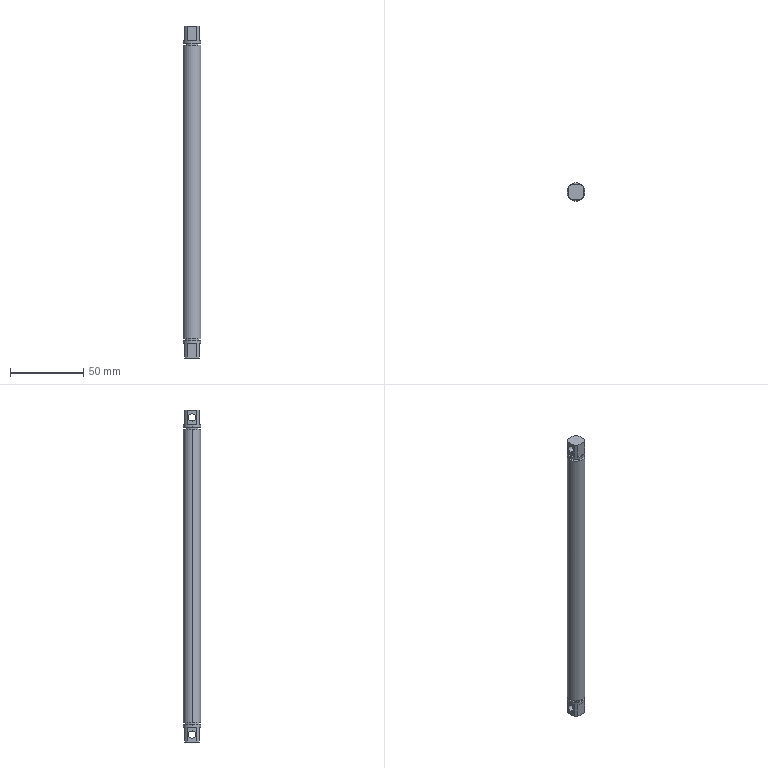Part | SolidWorks | features Extrusion 1, HoleWzd 1, ICE 1, MirrorPattern 1, RevCut 1 | 1 solid | 36 faces | box 12 x 12 x 226 mm | volume 24710 mm3 | plane 22 | cylinder 14 | commonest cylinder face diameters 12 x6 5 x4 8.691 x2 10.2 x2
STEP:
#1=CARTESIAN_POINT('',(5.,0.,110.5));
#2=VERTEX_POINT('',#1);
#3=CARTESIAN_POINT('',(5.,0.,105.5));
#4=VERTEX_POINT('',#3);
#5=CARTESIAN_POINT('',(5.,0.,108.));
#6=DIRECTION('',(1.,0.,0.));
#7=DIRECTION('',(0.,0.,-1.));
#8=AXIS2_PLACEMENT_3D('',#5,#6,#7);
#9=CIRCLE('',#8,2.5);
#10=EDGE_CURVE('',#2,#4,#9,.T.);
#11=ORIENTED_EDGE('',*,*,#10,.T.);
#12=CARTESIAN_POINT('',(-5.,0.,105.5));
#13=VERTEX_POINT('',#12);
#14=CARTESIAN_POINT('',(-5.,0.,105.5));
#15=DIRECTION('',(-1.,0.,0.));
#16=VECTOR('',#15,1000.);
#17=LINE('',#14,#16);
#18=EDGE_CURVE('',#4,#13,#17,.T.);
#19=ORIENTED_EDGE('',*,*,#18,.T.);
#20=CARTESIAN_POINT('',(-5.,0.,110.5));
#21=VERTEX_POINT('',#20);
#22=CARTESIAN_POINT('',(-5.,0.,108.));
#23=DIRECTION('',(-1.,0.,0.));
#24=DIRECTION('',(0.,0.,1.));
#25=AXIS2_PLACEMENT_3D('',#22,#23,#24);
#26=CIRCLE('',#25,2.5);
#27=EDGE_CURVE('',#13,#21,#26,.T.);
#28=ORIENTED_EDGE('',*,*,#27,.T.);
#29=CARTESIAN_POINT('',(-5.,0.,110.5));
#30=DIRECTION('',(-1.,0.,0.));
#31=VECTOR('',#30,1000.);
#32=LINE('',#29,#31);
#33=EDGE_CURVE('',#2,#21,#32,.T.);
#34=ORIENTED_EDGE('',*,*,#33,.F.);
#35=EDGE_LOOP('',(#11,#19,#28,#34));
#36=FACE_OUTER_BOUND('',#35,.T.);
#37=CARTESIAN_POINT('',(-5.,0.,108.));
#38=DIRECTION('',(-1.,0.,0.));
#39=DIRECTION('',(0.,0.,1.));
#40=AXIS2_PLACEMENT_3D('',#37,#38,#39);
#41=CYLINDRICAL_SURFACE('',#40,2.5);
#42=ADVANCED_FACE('',(#36),#41,.F.);
#43=CARTESIAN_POINT('',(5.,0.,-110.5));
#44=VERTEX_POINT('',#43);
#45=CARTESIAN_POINT('',(5.,0.,-105.5));
#46=VERTEX_POINT('',#45);
#47=CARTESIAN_POINT('',(5.,0.,-108.));
#48=DIRECTION('',(-1.,0.,0.));
#49=DIRECTION('',(0.,0.,1.));
#50=AXIS2_PLACEMENT_3D('',#47,#48,#49);
#51=CIRCLE('',#50,2.5);
#52=EDGE_CURVE('',#44,#46,#51,.T.);
#53=ORIENTED_EDGE('',*,*,#52,.F.);
#54=CARTESIAN_POINT('',(-5.,0.,-110.5));
#55=VERTEX_POINT('',#54);
#56=CARTESIAN_POINT('',(-5.,0.,-110.5));
#57=DIRECTION('',(-1.,0.,0.));
#58=VECTOR('',#57,1000.);
#59=LINE('',#56,#58);
#60=EDGE_CURVE('',#44,#55,#59,.T.);
#61=ORIENTED_EDGE('',*,*,#60,.T.);
#62=CARTESIAN_POINT('',(-5.,0.,-105.5));
#63=VERTEX_POINT('',#62);
#64=CARTESIAN_POINT('',(-5.,0.,-108.));
#65=DIRECTION('',(-1.,0.,0.));
#66=DIRECTION('',(0.,0.,1.));
#67=AXIS2_PLACEMENT_3D('',#64,#65,#66);
#68=CIRCLE('',#67,2.5);
#69=EDGE_CURVE('',#55,#63,#68,.T.);
#70=ORIENTED_EDGE('',*,*,#69,.T.);
#71=CARTESIAN_POINT('',(-5.,0.,-105.5));
#72=DIRECTION('',(-1.,0.,0.));
#73=VECTOR('',#72,1000.);
#74=LINE('',#71,#73);
#75=EDGE_CURVE('',#46,#63,#74,.T.);
#76=ORIENTED_EDGE('',*,*,#75,.F.);
#77=EDGE_LOOP('',(#53,#61,#70,#76));
#78=FACE_OUTER_BOUND('',#77,.T.);
#79=CARTESIAN_POINT('',(-5.,0.,-108.));
#80=DIRECTION('',(-1.,0.,0.));
#81=DIRECTION('',(0.,0.,1.));
#82=AXIS2_PLACEMENT_3D('',#79,#80,#81);
#83=CYLINDRICAL_SURFACE('',#82,2.5);
#84=ADVANCED_FACE('',(#78),#83,.F.);
#85=CARTESIAN_POINT('',(0.,-4.346,100.));
#86=VERTEX_POINT('',#85);
#87=CARTESIAN_POINT('',(0.,4.346,100.));
#88=VERTEX_POINT('',#87);
#89=CARTESIAN_POINT('',(0.,0.,100.));
#90=DIRECTION('',(0.,0.,1.));
#91=DIRECTION('',(0.,-1.,0.));
#92=AXIS2_PLACEMENT_3D('',#89,#90,#91);
#93=CIRCLE('',#92,4.346);
#94=EDGE_CURVE('',#86,#88,#93,.T.);
#95=ORIENTED_EDGE('',*,*,#94,.T.);
#96=CARTESIAN_POINT('',(0.,4.346,101.14));
#97=VERTEX_POINT('',#96);
#98=CARTESIAN_POINT('',(0.,4.346,0.));
#99=DIRECTION('',(0.,0.,1.));
#100=VECTOR('',#99,1000.);
#101=LINE('',#98,#100);
#102=EDGE_CURVE('',#88,#97,#101,.T.);
#103=ORIENTED_EDGE('',*,*,#102,.T.);
#104=CARTESIAN_POINT('',(0.,-4.346,101.14));
#105=VERTEX_POINT('',#104);
#106=CARTESIAN_POINT('',(0.,0.,101.14));
#107=DIRECTION('',(0.,0.,1.));
#108=DIRECTION('',(0.,-1.,0.));
#109=AXIS2_PLACEMENT_3D('',#106,#107,#108);
#110=CIRCLE('',#109,4.346);
#111=EDGE_CURVE('',#105,#97,#110,.T.);
#112=ORIENTED_EDGE('',*,*,#111,.F.);
#113=CARTESIAN_POINT('',(0.,-4.346,0.));
#114=DIRECTION('',(0.,0.,1.));
#115=VECTOR('',#114,1000.);
#116=LINE('',#113,#115);
#117=EDGE_CURVE('',#86,#105,#116,.T.);
#118=ORIENTED_EDGE('',*,*,#117,.F.);
#119=EDGE_LOOP('',(#95,#103,#112,#118));
#120=FACE_OUTER_BOUND('',#119,.T.);
#121=CARTESIAN_POINT('',(0.,0.,0.));
#122=DIRECTION('',(0.,0.,1.));
#123=DIRECTION('',(0.,-1.,0.));
#124=AXIS2_PLACEMENT_3D('',#121,#122,#123);
#125=CYLINDRICAL_SURFACE('',#124,4.346);
#126=ADVANCED_FACE('',(#120),#125,.T.);
#127=CARTESIAN_POINT('',(6.,0.,100.));
#128=VERTEX_POINT('',#127);
#129=CARTESIAN_POINT('',(-6.,0.,100.));
#130=VERTEX_POINT('',#129);
#131=CARTESIAN_POINT('',(0.,0.,100.));
#132=DIRECTION('',(0.,0.,1.));
#133=DIRECTION('',(0.,-1.,0.));
#134=AXIS2_PLACEMENT_3D('',#131,#132,#133);
#135=CIRCLE('',#134,6.);
#136=EDGE_CURVE('',#128,#130,#135,.T.);
#137=ORIENTED_EDGE('',*,*,#136,.F.);
#138=CARTESIAN_POINT('',(6.,0.,-100.));
#139=VERTEX_POINT('',#138);
#140=CARTESIAN_POINT('',(6.,0.,113.));
#141=DIRECTION('',(0.,0.,-1.));
#142=VECTOR('',#141,1000.);
#143=LINE('',#140,#142);
#144=EDGE_CURVE('',#128,#139,#143,.T.);
#145=ORIENTED_EDGE('',*,*,#144,.T.);
#146=CARTESIAN_POINT('',(-6.,0.,-100.));
#147=VERTEX_POINT('',#146);
#148=CARTESIAN_POINT('',(0.,0.,-100.));
#149=DIRECTION('',(0.,0.,1.));
#150=DIRECTION('',(0.,-1.,0.));
#151=AXIS2_PLACEMENT_3D('',#148,#149,#150);
#152=CIRCLE('',#151,6.);
#153=EDGE_CURVE('',#139,#147,#152,.T.);
#154=ORIENTED_EDGE('',*,*,#153,.T.);
#155=CARTESIAN_POINT('',(-6.,0.,113.));
#156=DIRECTION('',(0.,0.,-1.));
#157=VECTOR('',#156,1000.);
#158=LINE('',#155,#157);
#159=EDGE_CURVE('',#130,#147,#158,.T.);
#160=ORIENTED_EDGE('',*,*,#159,.F.);
#161=EDGE_LOOP('',(#137,#145,#154,#160));
#162=FACE_OUTER_BOUND('',#161,.T.);
#163=CARTESIAN_POINT('',(0.,0.,113.));
#164=DIRECTION('',(0.,0.,-1.));
#165=DIRECTION('',(-1.,0.,0.));
#166=AXIS2_PLACEMENT_3D('',#163,#164,#165);
#167=CYLINDRICAL_SURFACE('',#166,6.);
#168=ADVANCED_FACE('',(#162),#167,.T.);
#169=CARTESIAN_POINT('',(0.,-5.1,-101.14));
#170=VERTEX_POINT('',#169);
#171=CARTESIAN_POINT('',(0.,5.1,-101.14));
#172=VERTEX_POINT('',#171);
#173=CARTESIAN_POINT('',(0.,0.,-101.14));
#174=DIRECTION('',(0.,0.,1.));
#175=DIRECTION('',(0.,-1.,0.));
#176=AXIS2_PLACEMENT_3D('',#173,#174,#175);
#177=CIRCLE('',#176,5.1);
#178=EDGE_CURVE('',#170,#172,#177,.T.);
#179=ORIENTED_EDGE('',*,*,#178,.T.);
#180=CARTESIAN_POINT('',(0.,5.1,-100.));
#181=VERTEX_POINT('',#180);
#182=CARTESIAN_POINT('',(0.,5.1,0.));
#183=DIRECTION('',(0.,0.,1.));
#184=VECTOR('',#183,1000.);
#185=LINE('',#182,#184);
#186=EDGE_CURVE('',#172,#181,#185,.T.);
#187=ORIENTED_EDGE('',*,*,#186,.T.);
#188=CARTESIAN_POINT('',(0.,-5.1,-100.));
#189=VERTEX_POINT('',#188);
#190=CARTESIAN_POINT('',(0.,0.,-100.));
#191=DIRECTION('',(0.,0.,1.));
#192=DIRECTION('',(0.,-1.,0.));
#193=AXIS2_PLACEMENT_3D('',#190,#191,#192);
#194=CIRCLE('',#193,5.1);
#195=EDGE_CURVE('',#189,#181,#194,.T.);
#196=ORIENTED_EDGE('',*,*,#195,.F.);
#197=CARTESIAN_POINT('',(0.,-5.1,0.));
#198=DIRECTION('',(0.,0.,1.));
#199=VECTOR('',#198,1000.);
#200=LINE('',#197,#199);
#201=EDGE_CURVE('',#170,#189,#200,.T.);
#202=ORIENTED_EDGE('',*,*,#201,.F.);
#203=EDGE_LOOP('',(#179,#187,#196,#202));
#204=FACE_OUTER_BOUND('',#203,.T.);
#205=CARTESIAN_POINT('',(0.,0.,0.));
#206=DIRECTION('',(0.,0.,1.));
#207=DIRECTION('',(0.,-1.,0.));
#208=AXIS2_PLACEMENT_3D('',#205,#206,#207);
#209=CYLINDRICAL_SURFACE('',#208,5.1);
#210=ADVANCED_FACE('',(#204),#209,.T.);
#211=CARTESIAN_POINT('',(6.,0.,-101.14));
#212=VERTEX_POINT('',#211);
#213=CARTESIAN_POINT('',(-6.,0.,-101.14));
#214=VERTEX_POINT('',#213);
#215=CARTESIAN_POINT('',(0.,0.,-101.14));
#216=DIRECTION('',(0.,0.,1.));
#217=DIRECTION('',(0.,-1.,0.));
#218=AXIS2_PLACEMENT_3D('',#215,#216,#217);
#219=CIRCLE('',#218,6.);
#220=EDGE_CURVE('',#212,#214,#219,.T.);
#221=ORIENTED_EDGE('',*,*,#220,.F.);
#222=CARTESIAN_POINT('',(6.,0.,-103.));
#223=VERTEX_POINT('',#222);
#224=CARTESIAN_POINT('',(6.,0.,113.));
#225=DIRECTION('',(0.,0.,-1.));
#226=VECTOR('',#225,1000.);
#227=LINE('',#224,#226);
#228=EDGE_CURVE('',#212,#223,#227,.T.);
#229=ORIENTED_EDGE('',*,*,#228,.T.);
#230=CARTESIAN_POINT('',(5.,3.317,-103.));
#231=VERTEX_POINT('',#230);
#232=CARTESIAN_POINT('',(0.,0.,-103.));
#233=DIRECTION('',(0.,0.,-1.));
#234=DIRECTION('',(-1.,0.,0.));
#235=AXIS2_PLACEMENT_3D('',#232,#233,#234);
#236=CIRCLE('',#235,6.);
#237=EDGE_CURVE('',#231,#223,#236,.T.);
#238=ORIENTED_EDGE('',*,*,#237,.F.);
#239=CARTESIAN_POINT('',(5.,3.317,-113.));
#240=VERTEX_POINT('',#239);
#241=CARTESIAN_POINT('',(5.,3.317,-103.));
#242=DIRECTION('',(0.,0.,-1.));
#243=VECTOR('',#242,1000.);
#244=LINE('',#241,#243);
#245=EDGE_CURVE('',#231,#240,#244,.T.);
#246=ORIENTED_EDGE('',*,*,#245,.T.);
#247=CARTESIAN_POINT('',(3.317,5.,-113.));
#248=VERTEX_POINT('',#247);
#249=CARTESIAN_POINT('',(0.,0.,-113.));
#250=DIRECTION('',(0.,0.,1.));
#251=DIRECTION('',(1.,0.,0.));
#252=AXIS2_PLACEMENT_3D('',#249,#250,#251);
#253=CIRCLE('',#252,6.);
#254=EDGE_CURVE('',#240,#248,#253,.T.);
#255=ORIENTED_EDGE('',*,*,#254,.T.);
#256=CARTESIAN_POINT('',(3.317,5.,-103.));
#257=VERTEX_POINT('',#256);
#258=CARTESIAN_POINT('',(3.317,5.,-103.));
#259=DIRECTION('',(0.,0.,-1.));
#260=VECTOR('',#259,1000.);
#261=LINE('',#258,#260);
#262=EDGE_CURVE('',#257,#248,#261,.T.);
#263=ORIENTED_EDGE('',*,*,#262,.F.);
#264=CARTESIAN_POINT('',(-3.317,5.,-103.));
#265=VERTEX_POINT('',#264);
#266=CARTESIAN_POINT('',(0.,0.,-103.));
#267=DIRECTION('',(0.,0.,-1.));
#268=DIRECTION('',(-1.,0.,0.));
#269=AXIS2_PLACEMENT_3D('',#266,#267,#268);
#270=CIRCLE('',#269,6.);
#271=EDGE_CURVE('',#265,#257,#270,.T.);
#272=ORIENTED_EDGE('',*,*,#271,.F.);
#273=CARTESIAN_POINT('',(-3.317,5.,-113.));
#274=VERTEX_POINT('',#273);
#275=CARTESIAN_POINT('',(-3.317,5.,-103.));
#276=DIRECTION('',(0.,0.,-1.));
#277=VECTOR('',#276,1000.);
#278=LINE('',#275,#277);
#279=EDGE_CURVE('',#265,#274,#278,.T.);
#280=ORIENTED_EDGE('',*,*,#279,.T.);
#281=CARTESIAN_POINT('',(-5.,3.317,-113.));
#282=VERTEX_POINT('',#281);
#283=CARTESIAN_POINT('',(0.,0.,-113.));
#284=DIRECTION('',(0.,0.,1.));
#285=DIRECTION('',(1.,0.,0.));
#286=AXIS2_PLACEMENT_3D('',#283,#284,#285);
#287=CIRCLE('',#286,6.);
#288=EDGE_CURVE('',#274,#282,#287,.T.);
#289=ORIENTED_EDGE('',*,*,#288,.T.);
#290=CARTESIAN_POINT('',(-5.,3.317,-103.));
#291=VERTEX_POINT('',#290);
#292=CARTESIAN_POINT('',(-5.,3.317,-103.));
#293=DIRECTION('',(0.,0.,-1.));
#294=VECTOR('',#293,1000.);
#295=LINE('',#292,#294);
#296=EDGE_CURVE('',#291,#282,#295,.T.);
#297=ORIENTED_EDGE('',*,*,#296,.F.);
#298=CARTESIAN_POINT('',(-6.,0.,-103.));
#299=VERTEX_POINT('',#298);
#300=CARTESIAN_POINT('',(0.,0.,-103.));
#301=DIRECTION('',(0.,0.,-1.));
#302=DIRECTION('',(-1.,0.,0.));
#303=AXIS2_PLACEMENT_3D('',#300,#301,#302);
#304=CIRCLE('',#303,6.);
#305=EDGE_CURVE('',#299,#291,#304,.T.);
#306=ORIENTED_EDGE('',*,*,#305,.F.);
#307=CARTESIAN_POINT('',(-6.,0.,113.));
#308=DIRECTION('',(0.,0.,-1.));
#309=VECTOR('',#308,1000.);
#310=LINE('',#307,#309);
#311=EDGE_CURVE('',#214,#299,#310,.T.);
#312=ORIENTED_EDGE('',*,*,#311,.F.);
#313=EDGE_LOOP('',(#221,#229,#238,#246,#255,#263,#272,#280,#289,#297,#306,#312));
#314=FACE_OUTER_BOUND('',#313,.T.);
#315=CARTESIAN_POINT('',(0.,0.,113.));
#316=DIRECTION('',(0.,0.,-1.));
#317=DIRECTION('',(-1.,0.,0.));
#318=AXIS2_PLACEMENT_3D('',#315,#316,#317);
#319=CYLINDRICAL_SURFACE('',#318,6.);
#320=ADVANCED_FACE('',(#314),#319,.T.);
#321=CARTESIAN_POINT('',(5.,3.317,103.));
#322=VERTEX_POINT('',#321);
#323=CARTESIAN_POINT('',(6.,0.,103.));
#324=VERTEX_POINT('',#323);
#325=CARTESIAN_POINT('',(0.,0.,103.));
#326=DIRECTION('',(0.,0.,-1.));
#327=DIRECTION('',(-1.,0.,0.));
#328=AXIS2_PLACEMENT_3D('',#325,#326,#327);
#329=CIRCLE('',#328,6.);
#330=EDGE_CURVE('',#322,#324,#329,.T.);
#331=ORIENTED_EDGE('',*,*,#330,.T.);
#332=CARTESIAN_POINT('',(6.,0.,101.14));
#333=VERTEX_POINT('',#332);
#334=CARTESIAN_POINT('',(6.,0.,113.));
#335=DIRECTION('',(0.,0.,-1.));
#336=VECTOR('',#335,1000.);
#337=LINE('',#334,#336);
#338=EDGE_CURVE('',#324,#333,#337,.T.);
#339=ORIENTED_EDGE('',*,*,#338,.T.);
#340=CARTESIAN_POINT('',(-6.,0.,101.14));
#341=VERTEX_POINT('',#340);
#342=CARTESIAN_POINT('',(0.,0.,101.14));
#343=DIRECTION('',(0.,0.,1.));
#344=DIRECTION('',(0.,-1.,0.));
#345=AXIS2_PLACEMENT_3D('',#342,#343,#344);
#346=CIRCLE('',#345,6.);
#347=EDGE_CURVE('',#333,#341,#346,.T.);
#348=ORIENTED_EDGE('',*,*,#347,.T.);
#349=CARTESIAN_POINT('',(-6.,0.,103.));
#350=VERTEX_POINT('',#349);
#351=CARTESIAN_POINT('',(-6.,0.,113.));
#352=DIRECTION('',(0.,0.,-1.));
#353=VECTOR('',#352,1000.);
#354=LINE('',#351,#353);
#355=EDGE_CURVE('',#350,#341,#354,.T.);
#356=ORIENTED_EDGE('',*,*,#355,.F.);
#357=CARTESIAN_POINT('',(-5.,3.317,103.));
#358=VERTEX_POINT('',#357);
#359=CARTESIAN_POINT('',(0.,0.,103.));
#360=DIRECTION('',(0.,0.,-1.));
#361=DIRECTION('',(-1.,0.,0.));
#362=AXIS2_PLACEMENT_3D('',#359,#360,#361);
#363=CIRCLE('',#362,6.);
#364=EDGE_CURVE('',#350,#358,#363,.T.);
#365=ORIENTED_EDGE('',*,*,#364,.T.);
#366=CARTESIAN_POINT('',(-5.,3.317,113.));
#367=VERTEX_POINT('',#366);
#368=CARTESIAN_POINT('',(-5.,3.317,103.));
#369=DIRECTION('',(0.,0.,1.));
#370=VECTOR('',#369,1000.);
#371=LINE('',#368,#370);
#372=EDGE_CURVE('',#358,#367,#371,.T.);
#373=ORIENTED_EDGE('',*,*,#372,.T.);
#374=CARTESIAN_POINT('',(-3.317,5.,113.));
#375=VERTEX_POINT('',#374);
#376=CARTESIAN_POINT('',(0.,0.,113.));
#377=DIRECTION('',(0.,0.,1.));
#378=DIRECTION('',(1.,0.,0.));
#379=AXIS2_PLACEMENT_3D('',#376,#377,#378);
#380=CIRCLE('',#379,6.);
#381=EDGE_CURVE('',#375,#367,#380,.T.);
#382=ORIENTED_EDGE('',*,*,#381,.F.);
#383=CARTESIAN_POINT('',(-3.317,5.,103.));
#384=VERTEX_POINT('',#383);
#385=CARTESIAN_POINT('',(-3.317,5.,103.));
#386=DIRECTION('',(0.,0.,1.));
#387=VECTOR('',#386,1000.);
#388=LINE('',#385,#387);
#389=EDGE_CURVE('',#384,#375,#388,.T.);
#390=ORIENTED_EDGE('',*,*,#389,.F.);
#391=CARTESIAN_POINT('',(3.317,5.,103.));
#392=VERTEX_POINT('',#391);
#393=CARTESIAN_POINT('',(0.,0.,103.));
#394=DIRECTION('',(0.,0.,-1.));
#395=DIRECTION('',(-1.,0.,0.));
#396=AXIS2_PLACEMENT_3D('',#393,#394,#395);
#397=CIRCLE('',#396,6.);
#398=EDGE_CURVE('',#384,#392,#397,.T.);
#399=ORIENTED_EDGE('',*,*,#398,.T.);
#400=CARTESIAN_POINT('',(3.317,5.,113.));
#401=VERTEX_POINT('',#400);
#402=CARTESIAN_POINT('',(3.317,5.,103.));
#403=DIRECTION('',(0.,0.,1.));
#404=VECTOR('',#403,1000.);
#405=LINE('',#402,#404);
#406=EDGE_CURVE('',#392,#401,#405,.T.);
#407=ORIENTED_EDGE('',*,*,#406,.T.);
#408=CARTESIAN_POINT('',(5.,3.317,113.));
#409=VERTEX_POINT('',#408);
#410=CARTESIAN_POINT('',(0.,0.,113.));
#411=DIRECTION('',(0.,0.,1.));
#412=DIRECTION('',(1.,0.,0.));
#413=AXIS2_PLACEMENT_3D('',#410,#411,#412);
#414=CIRCLE('',#413,6.);
#415=EDGE_CURVE('',#409,#401,#414,.T.);
#416=ORIENTED_EDGE('',*,*,#415,.F.);
#417=CARTESIAN_POINT('',(5.,3.317,103.));
#418=DIRECTION('',(0.,0.,1.));
#419=VECTOR('',#418,1000.);
#420=LINE('',#417,#419);
#421=EDGE_CURVE('',#322,#409,#420,.T.);
#422=ORIENTED_EDGE('',*,*,#421,.F.);
#423=EDGE_LOOP('',(#331,#339,#348,#356,#365,#373,#382,#390,#399,#407,#416,#422));
#424=FACE_OUTER_BOUND('',#423,.T.);
#425=CARTESIAN_POINT('',(0.,0.,113.));
#426=DIRECTION('',(0.,0.,-1.));
#427=DIRECTION('',(-1.,0.,0.));
#428=AXIS2_PLACEMENT_3D('',#425,#426,#427);
#429=CYLINDRICAL_SURFACE('',#428,6.);
#430=ADVANCED_FACE('',(#424),#429,.T.);
#431=CARTESIAN_POINT('',(3.317,-5.,113.));
#432=VERTEX_POINT('',#431);
#433=CARTESIAN_POINT('',(5.,-3.317,113.));
#434=VERTEX_POINT('',#433);
#435=CARTESIAN_POINT('',(0.,0.,113.));
#436=DIRECTION('',(0.,0.,1.));
#437=DIRECTION('',(1.,0.,0.));
#438=AXIS2_PLACEMENT_3D('',#435,#436,#437);
#439=CIRCLE('',#438,6.);
#440=EDGE_CURVE('',#432,#434,#439,.T.);
#441=ORIENTED_EDGE('',*,*,#440,.T.);
#442=CARTESIAN_POINT('',(5.,3.317,113.));
#443=DIRECTION('',(0.,1.,0.));
#444=VECTOR('',#443,1000.);
#445=LINE('',#442,#444);
#446=EDGE_CURVE('',#434,#409,#445,.T.);
#447=ORIENTED_EDGE('',*,*,#446,.T.);
#448=ORIENTED_EDGE('',*,*,#415,.T.);
#449=CARTESIAN_POINT('',(3.317,5.,113.));
#450=DIRECTION('',(-1.,0.,0.));
#451=VECTOR('',#450,1000.);
#452=LINE('',#449,#451);
#453=EDGE_CURVE('',#401,#375,#452,.T.);
#454=ORIENTED_EDGE('',*,*,#453,.T.);
#455=ORIENTED_EDGE('',*,*,#381,.T.);
#456=CARTESIAN_POINT('',(-5.,-3.317,113.));
#457=VERTEX_POINT('',#456);
#458=CARTESIAN_POINT('',(-5.,3.317,113.));
#459=DIRECTION('',(0.,-1.,0.));
#460=VECTOR('',#459,1000.);
#461=LINE('',#458,#460);
#462=EDGE_CURVE('',#367,#457,#461,.T.);
#463=ORIENTED_EDGE('',*,*,#462,.T.);
#464=CARTESIAN_POINT('',(-3.317,-5.,113.));
#465=VERTEX_POINT('',#464);
#466=CARTESIAN_POINT('',(0.,0.,113.));
#467=DIRECTION('',(0.,0.,1.));
#468=DIRECTION('',(1.,0.,0.));
#469=AXIS2_PLACEMENT_3D('',#466,#467,#468);
#470=CIRCLE('',#469,6.);
#471=EDGE_CURVE('',#457,#465,#470,.T.);
#472=ORIENTED_EDGE('',*,*,#471,.T.);
#473=CARTESIAN_POINT('',(-3.317,-5.,113.));
#474=DIRECTION('',(1.,0.,0.));
#475=VECTOR('',#474,1000.);
#476=LINE('',#473,#475);
#477=EDGE_CURVE('',#465,#432,#476,.T.);
#478=ORIENTED_EDGE('',*,*,#477,.T.);
#479=EDGE_LOOP('',(#441,#447,#448,#454,#455,#463,#472,#478));
#480=FACE_OUTER_BOUND('',#479,.T.);
#481=CARTESIAN_POINT('',(0.,0.,113.));
#482=DIRECTION('',(0.,0.,1.));
#483=DIRECTION('',(1.,0.,0.));
#484=AXIS2_PLACEMENT_3D('',#481,#482,#483);
#485=PLANE('',#484);
#486=ADVANCED_FACE('',(#480),#485,.T.);
#487=ORIENTED_EDGE('',*,*,#338,.F.);
#488=CARTESIAN_POINT('',(5.,-3.317,103.));
#489=VERTEX_POINT('',#488);
#490=CARTESIAN_POINT('',(0.,0.,103.));
#491=DIRECTION('',(0.,0.,-1.));
#492=DIRECTION('',(-1.,0.,0.));
#493=AXIS2_PLACEMENT_3D('',#490,#491,#492);
#494=CIRCLE('',#493,6.);
#495=EDGE_CURVE('',#324,#489,#494,.T.);
#496=ORIENTED_EDGE('',*,*,#495,.T.);
#497=CARTESIAN_POINT('',(5.,-3.317,103.));
#498=DIRECTION('',(0.,0.,1.));
#499=VECTOR('',#498,1000.);
#500=LINE('',#497,#499);
#501=EDGE_CURVE('',#489,#434,#500,.T.);
#502=ORIENTED_EDGE('',*,*,#501,.T.);
#503=ORIENTED_EDGE('',*,*,#440,.F.);
#504=CARTESIAN_POINT('',(3.317,-5.,103.));
#505=VERTEX_POINT('',#504);
#506=CARTESIAN_POINT('',(3.317,-5.,103.));
#507=DIRECTION('',(0.,0.,1.));
#508=VECTOR('',#507,1000.);
#509=LINE('',#506,#508);
#510=EDGE_CURVE('',#505,#432,#509,.T.);
#511=ORIENTED_EDGE('',*,*,#510,.F.);
#512=CARTESIAN_POINT('',(-3.317,-5.,103.));
#513=VERTEX_POINT('',#512);
#514=CARTESIAN_POINT('',(0.,0.,103.));
#515=DIRECTION('',(0.,0.,-1.));
#516=DIRECTION('',(-1.,0.,0.));
#517=AXIS2_PLACEMENT_3D('',#514,#515,#516);
#518=CIRCLE('',#517,6.);
#519=EDGE_CURVE('',#505,#513,#518,.T.);
#520=ORIENTED_EDGE('',*,*,#519,.T.);
#521=CARTESIAN_POINT('',(-3.317,-5.,103.));
#522=DIRECTION('',(0.,0.,1.));
#523=VECTOR('',#522,1000.);
#524=LINE('',#521,#523);
#525=EDGE_CURVE('',#513,#465,#524,.T.);
#526=ORIENTED_EDGE('',*,*,#525,.T.);
#527=ORIENTED_EDGE('',*,*,#471,.F.);
#528=CARTESIAN_POINT('',(-5.,-3.317,103.));
#529=VERTEX_POINT('',#528);
#530=CARTESIAN_POINT('',(-5.,-3.317,103.));
#531=DIRECTION('',(0.,0.,1.));
#532=VECTOR('',#531,1000.);
#533=LINE('',#530,#532);
#534=EDGE_CURVE('',#529,#457,#533,.T.);
#535=ORIENTED_EDGE('',*,*,#534,.F.);
#536=CARTESIAN_POINT('',(0.,0.,103.));
#537=DIRECTION('',(0.,0.,-1.));
#538=DIRECTION('',(-1.,0.,0.));
#539=AXIS2_PLACEMENT_3D('',#536,#537,#538);
#540=CIRCLE('',#539,6.);
#541=EDGE_CURVE('',#529,#350,#540,.T.);
#542=ORIENTED_EDGE('',*,*,#541,.T.);
#543=ORIENTED_EDGE('',*,*,#355,.T.);
#544=CARTESIAN_POINT('',(0.,0.,101.14));
#545=DIRECTION('',(0.,0.,1.));
#546=DIRECTION('',(0.,-1.,0.));
#547=AXIS2_PLACEMENT_3D('',#544,#545,#546);
#548=CIRCLE('',#547,6.);
#549=EDGE_CURVE('',#341,#333,#548,.T.);
#550=ORIENTED_EDGE('',*,*,#549,.T.);
#551=EDGE_LOOP('',(#487,#496,#502,#503,#511,#520,#526,#527,#535,#542,#543,#550));
#552=FACE_OUTER_BOUND('',#551,.T.);
#553=CARTESIAN_POINT('',(0.,0.,113.));
#554=DIRECTION('',(0.,0.,-1.));
#555=DIRECTION('',(-1.,0.,0.));
#556=AXIS2_PLACEMENT_3D('',#553,#554,#555);
#557=CYLINDRICAL_SURFACE('',#556,6.);
#558=ADVANCED_FACE('',(#552),#557,.T.);
#559=ORIENTED_EDGE('',*,*,#228,.F.);
#560=CARTESIAN_POINT('',(0.,0.,-101.14));
#561=DIRECTION('',(0.,0.,1.));
#562=DIRECTION('',(0.,-1.,0.));
#563=AXIS2_PLACEMENT_3D('',#560,#561,#562);
#564=CIRCLE('',#563,6.);
#565=EDGE_CURVE('',#214,#212,#564,.T.);
#566=ORIENTED_EDGE('',*,*,#565,.F.);
#567=ORIENTED_EDGE('',*,*,#311,.T.);
#568=CARTESIAN_POINT('',(-5.,-3.317,-103.));
#569=VERTEX_POINT('',#568);
#570=CARTESIAN_POINT('',(0.,0.,-103.));
#571=DIRECTION('',(0.,0.,-1.));
#572=DIRECTION('',(-1.,0.,0.));
#573=AXIS2_PLACEMENT_3D('',#570,#571,#572);
#574=CIRCLE('',#573,6.);
#575=EDGE_CURVE('',#569,#299,#574,.T.);
#576=ORIENTED_EDGE('',*,*,#575,.F.);
#577=CARTESIAN_POINT('',(-5.,-3.317,-113.));
#578=VERTEX_POINT('',#577);
#579=CARTESIAN_POINT('',(-5.,-3.317,-103.));
#580=DIRECTION('',(0.,0.,-1.));
#581=VECTOR('',#580,1000.);
#582=LINE('',#579,#581);
#583=EDGE_CURVE('',#569,#578,#582,.T.);
#584=ORIENTED_EDGE('',*,*,#583,.T.);
#585=CARTESIAN_POINT('',(-3.317,-5.,-113.));
#586=VERTEX_POINT('',#585);
#587=CARTESIAN_POINT('',(0.,0.,-113.));
#588=DIRECTION('',(0.,0.,1.));
#589=DIRECTION('',(1.,0.,0.));
#590=AXIS2_PLACEMENT_3D('',#587,#588,#589);
#591=CIRCLE('',#590,6.);
#592=EDGE_CURVE('',#578,#586,#591,.T.);
#593=ORIENTED_EDGE('',*,*,#592,.T.);
#594=CARTESIAN_POINT('',(-3.317,-5.,-103.));
#595=VERTEX_POINT('',#594);
#596=CARTESIAN_POINT('',(-3.317,-5.,-103.));
#597=DIRECTION('',(0.,0.,-1.));
#598=VECTOR('',#597,1000.);
#599=LINE('',#596,#598);
#600=EDGE_CURVE('',#595,#586,#599,.T.);
#601=ORIENTED_EDGE('',*,*,#600,.F.);
#602=CARTESIAN_POINT('',(3.317,-5.,-103.));
#603=VERTEX_POINT('',#602);
#604=CARTESIAN_POINT('',(0.,0.,-103.));
#605=DIRECTION('',(0.,0.,-1.));
#606=DIRECTION('',(-1.,0.,0.));
#607=AXIS2_PLACEMENT_3D('',#604,#605,#606);
#608=CIRCLE('',#607,6.);
#609=EDGE_CURVE('',#603,#595,#608,.T.);
#610=ORIENTED_EDGE('',*,*,#609,.F.);
#611=CARTESIAN_POINT('',(3.317,-5.,-113.));
#612=VERTEX_POINT('',#611);
#613=CARTESIAN_POINT('',(3.317,-5.,-103.));
#614=DIRECTION('',(0.,0.,-1.));
#615=VECTOR('',#614,1000.);
#616=LINE('',#613,#615);
#617=EDGE_CURVE('',#603,#612,#616,.T.);
#618=ORIENTED_EDGE('',*,*,#617,.T.);
#619=CARTESIAN_POINT('',(5.,-3.317,-113.));
#620=VERTEX_POINT('',#619);
#621=CARTESIAN_POINT('',(0.,0.,-113.));
#622=DIRECTION('',(0.,0.,1.));
#623=DIRECTION('',(1.,0.,0.));
#624=AXIS2_PLACEMENT_3D('',#621,#622,#623);
#625=CIRCLE('',#624,6.);
#626=EDGE_CURVE('',#612,#620,#625,.T.);
#627=ORIENTED_EDGE('',*,*,#626,.T.);
#628=CARTESIAN_POINT('',(5.,-3.317,-103.));
#629=VERTEX_POINT('',#628);
#630=CARTESIAN_POINT('',(5.,-3.317,-103.));
#631=DIRECTION('',(0.,0.,-1.));
#632=VECTOR('',#631,1000.);
#633=LINE('',#630,#632);
#634=EDGE_CURVE('',#629,#620,#633,.T.);
#635=ORIENTED_EDGE('',*,*,#634,.F.);
#636=CARTESIAN_POINT('',(0.,0.,-103.));
#637=DIRECTION('',(0.,0.,-1.));
#638=DIRECTION('',(-1.,0.,0.));
#639=AXIS2_PLACEMENT_3D('',#636,#637,#638);
#640=CIRCLE('',#639,6.);
#641=EDGE_CURVE('',#223,#629,#640,.T.);
#642=ORIENTED_EDGE('',*,*,#641,.F.);
#643=EDGE_LOOP('',(#559,#566,#567,#576,#584,#593,#601,#610,#618,#627,#635,#642));
#644=FACE_OUTER_BOUND('',#643,.T.);
#645=CARTESIAN_POINT('',(0.,0.,113.));
#646=DIRECTION('',(0.,0.,-1.));
#647=DIRECTION('',(-1.,0.,0.));
#648=AXIS2_PLACEMENT_3D('',#645,#646,#647);
#649=CYLINDRICAL_SURFACE('',#648,6.);
#650=ADVANCED_FACE('',(#644),#649,.T.);
#651=ORIENTED_EDGE('',*,*,#254,.F.);
#652=CARTESIAN_POINT('',(5.,3.317,-113.));
#653=DIRECTION('',(0.,1.,0.));
#654=VECTOR('',#653,1000.);
#655=LINE('',#652,#654);
#656=EDGE_CURVE('',#620,#240,#655,.T.);
#657=ORIENTED_EDGE('',*,*,#656,.F.);
#658=ORIENTED_EDGE('',*,*,#626,.F.);
#659=CARTESIAN_POINT('',(-3.317,-5.,-113.));
#660=DIRECTION('',(1.,0.,0.));
#661=VECTOR('',#660,1000.);
#662=LINE('',#659,#661);
#663=EDGE_CURVE('',#586,#612,#662,.T.);
#664=ORIENTED_EDGE('',*,*,#663,.F.);
#665=ORIENTED_EDGE('',*,*,#592,.F.);
#666=CARTESIAN_POINT('',(-5.,3.317,-113.));
#667=DIRECTION('',(0.,-1.,0.));
#668=VECTOR('',#667,1000.);
#669=LINE('',#666,#668);
#670=EDGE_CURVE('',#282,#578,#669,.T.);
#671=ORIENTED_EDGE('',*,*,#670,.F.);
#672=ORIENTED_EDGE('',*,*,#288,.F.);
#673=CARTESIAN_POINT('',(3.317,5.,-113.));
#674=DIRECTION('',(-1.,0.,0.));
#675=VECTOR('',#674,1000.);
#676=LINE('',#673,#675);
#677=EDGE_CURVE('',#248,#274,#676,.T.);
#678=ORIENTED_EDGE('',*,*,#677,.F.);
#679=EDGE_LOOP('',(#651,#657,#658,#664,#665,#671,#672,#678));
#680=FACE_OUTER_BOUND('',#679,.T.);
#681=CARTESIAN_POINT('',(0.,0.,-113.));
#682=DIRECTION('',(0.,0.,1.));
#683=DIRECTION('',(1.,0.,0.));
#684=AXIS2_PLACEMENT_3D('',#681,#682,#683);
#685=PLANE('',#684);
#686=ADVANCED_FACE('',(#680),#685,.F.);
#687=ORIENTED_EDGE('',*,*,#565,.T.);
#688=ORIENTED_EDGE('',*,*,#220,.T.);
#689=EDGE_LOOP('',(#687,#688));
#690=FACE_OUTER_BOUND('',#689,.T.);
#691=ORIENTED_EDGE('',*,*,#178,.F.);
#692=CARTESIAN_POINT('',(0.,0.,-101.14));
#693=DIRECTION('',(0.,0.,1.));
#694=DIRECTION('',(0.,-1.,0.));
#695=AXIS2_PLACEMENT_3D('',#692,#693,#694);
#696=CIRCLE('',#695,5.1);
#697=EDGE_CURVE('',#172,#170,#696,.T.);
#698=ORIENTED_EDGE('',*,*,#697,.F.);
#699=EDGE_LOOP('',(#691,#698));
#700=FACE_BOUND('',#699,.T.);
#701=CARTESIAN_POINT('',(0.,6.,-101.14));
#702=DIRECTION('',(0.,0.,1.));
#703=DIRECTION('',(0.,-1.,0.));
#704=AXIS2_PLACEMENT_3D('',#701,#702,#703);
#705=PLANE('',#704);
#706=ADVANCED_FACE('',(#690,#700),#705,.T.);
#707=ORIENTED_EDGE('',*,*,#186,.F.);
#708=ORIENTED_EDGE('',*,*,#697,.T.);
#709=ORIENTED_EDGE('',*,*,#201,.T.);
#710=CARTESIAN_POINT('',(0.,0.,-100.));
#711=DIRECTION('',(0.,0.,1.));
#712=DIRECTION('',(0.,-1.,0.));
#713=AXIS2_PLACEMENT_3D('',#710,#711,#712);
#714=CIRCLE('',#713,5.1);
#715=EDGE_CURVE('',#181,#189,#714,.T.);
#716=ORIENTED_EDGE('',*,*,#715,.F.);
#717=EDGE_LOOP('',(#707,#708,#709,#716));
#718=FACE_OUTER_BOUND('',#717,.T.);
#719=CARTESIAN_POINT('',(0.,0.,0.));
#720=DIRECTION('',(0.,0.,1.));
#721=DIRECTION('',(0.,-1.,0.));
#722=AXIS2_PLACEMENT_3D('',#719,#720,#721);
#723=CYLINDRICAL_SURFACE('',#722,5.1);
#724=ADVANCED_FACE('',(#718),#723,.T.);
#725=ORIENTED_EDGE('',*,*,#195,.T.);
#726=ORIENTED_EDGE('',*,*,#715,.T.);
#727=EDGE_LOOP('',(#725,#726));
#728=FACE_BOUND('',#727,.T.);
#729=CARTESIAN_POINT('',(0.,0.,-100.));
#730=DIRECTION('',(0.,0.,1.));
#731=DIRECTION('',(0.,-1.,0.));
#732=AXIS2_PLACEMENT_3D('',#729,#730,#731);
#733=CIRCLE('',#732,6.);
#734=EDGE_CURVE('',#147,#139,#733,.T.);
#735=ORIENTED_EDGE('',*,*,#734,.F.);
#736=ORIENTED_EDGE('',*,*,#153,.F.);
#737=EDGE_LOOP('',(#735,#736));
#738=FACE_OUTER_BOUND('',#737,.T.);
#739=CARTESIAN_POINT('',(0.,6.,-100.));
#740=DIRECTION('',(0.,0.,-1.));
#741=DIRECTION('',(0.,1.,0.));
#742=AXIS2_PLACEMENT_3D('',#739,#740,#741);
#743=PLANE('',#742);
#744=ADVANCED_FACE('',(#728,#738),#743,.T.);
#745=ORIENTED_EDGE('',*,*,#144,.F.);
#746=CARTESIAN_POINT('',(0.,0.,100.));
#747=DIRECTION('',(0.,0.,1.));
#748=DIRECTION('',(0.,-1.,0.));
#749=AXIS2_PLACEMENT_3D('',#746,#747,#748);
#750=CIRCLE('',#749,6.);
#751=EDGE_CURVE('',#130,#128,#750,.T.);
#752=ORIENTED_EDGE('',*,*,#751,.F.);
#753=ORIENTED_EDGE('',*,*,#159,.T.);
#754=ORIENTED_EDGE('',*,*,#734,.T.);
#755=EDGE_LOOP('',(#745,#752,#753,#754));
#756=FACE_OUTER_BOUND('',#755,.T.);
#757=CARTESIAN_POINT('',(0.,0.,113.));
#758=DIRECTION('',(0.,0.,-1.));
#759=DIRECTION('',(-1.,0.,0.));
#760=AXIS2_PLACEMENT_3D('',#757,#758,#759);
#761=CYLINDRICAL_SURFACE('',#760,6.);
#762=ADVANCED_FACE('',(#756),#761,.T.);
#763=ORIENTED_EDGE('',*,*,#751,.T.);
#764=ORIENTED_EDGE('',*,*,#136,.T.);
#765=EDGE_LOOP('',(#763,#764));
#766=FACE_OUTER_BOUND('',#765,.T.);
#767=ORIENTED_EDGE('',*,*,#94,.F.);
#768=CARTESIAN_POINT('',(0.,0.,100.));
#769=DIRECTION('',(0.,0.,1.));
#770=DIRECTION('',(0.,-1.,0.));
#771=AXIS2_PLACEMENT_3D('',#768,#769,#770);
#772=CIRCLE('',#771,4.346);
#773=EDGE_CURVE('',#88,#86,#772,.T.);
#774=ORIENTED_EDGE('',*,*,#773,.F.);
#775=EDGE_LOOP('',(#767,#774));
#776=FACE_BOUND('',#775,.T.);
#777=CARTESIAN_POINT('',(0.,6.,100.));
#778=DIRECTION('',(0.,0.,1.));
#779=DIRECTION('',(0.,-1.,0.));
#780=AXIS2_PLACEMENT_3D('',#777,#778,#779);
#781=PLANE('',#780);
#782=ADVANCED_FACE('',(#766,#776),#781,.T.);
#783=ORIENTED_EDGE('',*,*,#102,.F.);
#784=ORIENTED_EDGE('',*,*,#773,.T.);
#785=ORIENTED_EDGE('',*,*,#117,.T.);
#786=CARTESIAN_POINT('',(0.,0.,101.14));
#787=DIRECTION('',(0.,0.,1.));
#788=DIRECTION('',(0.,-1.,0.));
#789=AXIS2_PLACEMENT_3D('',#786,#787,#788);
#790=CIRCLE('',#789,4.346);
#791=EDGE_CURVE('',#97,#105,#790,.T.);
#792=ORIENTED_EDGE('',*,*,#791,.F.);
#793=EDGE_LOOP('',(#783,#784,#785,#792));
#794=FACE_OUTER_BOUND('',#793,.T.);
#795=CARTESIAN_POINT('',(0.,0.,0.));
#796=DIRECTION('',(0.,0.,1.));
#797=DIRECTION('',(0.,-1.,0.));
#798=AXIS2_PLACEMENT_3D('',#795,#796,#797);
#799=CYLINDRICAL_SURFACE('',#798,4.346);
#800=ADVANCED_FACE('',(#794),#799,.T.);
#801=ORIENTED_EDGE('',*,*,#111,.T.);
#802=ORIENTED_EDGE('',*,*,#791,.T.);
#803=EDGE_LOOP('',(#801,#802));
#804=FACE_BOUND('',#803,.T.);
#805=ORIENTED_EDGE('',*,*,#549,.F.);
#806=ORIENTED_EDGE('',*,*,#347,.F.);
#807=EDGE_LOOP('',(#805,#806));
#808=FACE_OUTER_BOUND('',#807,.T.);
#809=CARTESIAN_POINT('',(0.,6.,101.14));
#810=DIRECTION('',(0.,0.,-1.));
#811=DIRECTION('',(0.,1.,0.));
#812=AXIS2_PLACEMENT_3D('',#809,#810,#811);
#813=PLANE('',#812);
#814=ADVANCED_FACE('',(#804,#808),#813,.T.);
#815=ORIENTED_EDGE('',*,*,#663,.T.);
#816=ORIENTED_EDGE('',*,*,#617,.F.);
#817=CARTESIAN_POINT('',(-3.317,-5.,-103.));
#818=DIRECTION('',(1.,0.,0.));
#819=VECTOR('',#818,1000.);
#820=LINE('',#817,#819);
#821=EDGE_CURVE('',#595,#603,#820,.T.);
#822=ORIENTED_EDGE('',*,*,#821,.F.);
#823=ORIENTED_EDGE('',*,*,#600,.T.);
#824=EDGE_LOOP('',(#815,#816,#822,#823));
#825=FACE_OUTER_BOUND('',#824,.T.);
#826=CARTESIAN_POINT('',(-3.317,-5.,-103.));
#827=DIRECTION('',(0.,1.,0.));
#828=DIRECTION('',(0.,0.,1.));
#829=AXIS2_PLACEMENT_3D('',#826,#827,#828);
#830=PLANE('',#829);
#831=ADVANCED_FACE('',(#825),#830,.F.);
#832=ORIENTED_EDGE('',*,*,#609,.T.);
#833=ORIENTED_EDGE('',*,*,#821,.T.);
#834=EDGE_LOOP('',(#832,#833));
#835=FACE_OUTER_BOUND('',#834,.T.);
#836=CARTESIAN_POINT('',(0.,0.,-103.));
#837=DIRECTION('',(0.,0.,-1.));
#838=DIRECTION('',(-1.,0.,0.));
#839=AXIS2_PLACEMENT_3D('',#836,#837,#838);
#840=PLANE('',#839);
#841=ADVANCED_FACE('',(#835),#840,.T.);
#842=ORIENTED_EDGE('',*,*,#677,.T.);
#843=ORIENTED_EDGE('',*,*,#279,.F.);
#844=CARTESIAN_POINT('',(3.317,5.,-103.));
#845=DIRECTION('',(-1.,0.,0.));
#846=VECTOR('',#845,1000.);
#847=LINE('',#844,#846);
#848=EDGE_CURVE('',#257,#265,#847,.T.);
#849=ORIENTED_EDGE('',*,*,#848,.F.);
#850=ORIENTED_EDGE('',*,*,#262,.T.);
#851=EDGE_LOOP('',(#842,#843,#849,#850));
#852=FACE_OUTER_BOUND('',#851,.T.);
#853=CARTESIAN_POINT('',(3.317,5.,-103.));
#854=DIRECTION('',(0.,-1.,0.));
#855=DIRECTION('',(0.,0.,-1.));
#856=AXIS2_PLACEMENT_3D('',#853,#854,#855);
#857=PLANE('',#856);
#858=ADVANCED_FACE('',(#852),#857,.F.);
#859=ORIENTED_EDGE('',*,*,#271,.T.);
#860=ORIENTED_EDGE('',*,*,#848,.T.);
#861=EDGE_LOOP('',(#859,#860));
#862=FACE_OUTER_BOUND('',#861,.T.);
#863=CARTESIAN_POINT('',(0.,0.,-103.));
#864=DIRECTION('',(0.,0.,-1.));
#865=DIRECTION('',(-1.,0.,0.));
#866=AXIS2_PLACEMENT_3D('',#863,#864,#865);
#867=PLANE('',#866);
#868=ADVANCED_FACE('',(#862),#867,.T.);
#869=CARTESIAN_POINT('',(-5.,0.,-108.));
#870=DIRECTION('',(-1.,0.,0.));
#871=DIRECTION('',(0.,0.,1.));
#872=AXIS2_PLACEMENT_3D('',#869,#870,#871);
#873=CIRCLE('',#872,2.5);
#874=EDGE_CURVE('',#63,#55,#873,.T.);
#875=ORIENTED_EDGE('',*,*,#874,.F.);
#876=ORIENTED_EDGE('',*,*,#69,.F.);
#877=EDGE_LOOP('',(#875,#876));
#878=FACE_BOUND('',#877,.T.);
#879=ORIENTED_EDGE('',*,*,#670,.T.);
#880=ORIENTED_EDGE('',*,*,#583,.F.);
#881=CARTESIAN_POINT('',(-5.,3.317,-103.));
#882=DIRECTION('',(0.,-1.,0.));
#883=VECTOR('',#882,1000.);
#884=LINE('',#881,#883);
#885=EDGE_CURVE('',#291,#569,#884,.T.);
#886=ORIENTED_EDGE('',*,*,#885,.F.);
#887=ORIENTED_EDGE('',*,*,#296,.T.);
#888=EDGE_LOOP('',(#879,#880,#886,#887));
#889=FACE_OUTER_BOUND('',#888,.T.);
#890=CARTESIAN_POINT('',(-5.,3.317,-103.));
#891=DIRECTION('',(1.,0.,0.));
#892=DIRECTION('',(0.,0.,-1.));
#893=AXIS2_PLACEMENT_3D('',#890,#891,#892);
#894=PLANE('',#893);
#895=ADVANCED_FACE('',(#878,#889),#894,.F.);
#896=ORIENTED_EDGE('',*,*,#575,.T.);
#897=ORIENTED_EDGE('',*,*,#305,.T.);
#898=ORIENTED_EDGE('',*,*,#885,.T.);
#899=EDGE_LOOP('',(#896,#897,#898));
#900=FACE_OUTER_BOUND('',#899,.T.);
#901=CARTESIAN_POINT('',(0.,0.,-103.));
#902=DIRECTION('',(0.,0.,-1.));
#903=DIRECTION('',(-1.,0.,0.));
#904=AXIS2_PLACEMENT_3D('',#901,#902,#903);
#905=PLANE('',#904);
#906=ADVANCED_FACE('',(#900),#905,.T.);
#907=CARTESIAN_POINT('',(5.,0.,-108.));
#908=DIRECTION('',(-1.,0.,0.));
#909=DIRECTION('',(0.,0.,1.));
#910=AXIS2_PLACEMENT_3D('',#907,#908,#909);
#911=CIRCLE('',#910,2.5);
#912=EDGE_CURVE('',#46,#44,#911,.T.);
#913=ORIENTED_EDGE('',*,*,#912,.T.);
#914=ORIENTED_EDGE('',*,*,#52,.T.);
#915=EDGE_LOOP('',(#913,#914));
#916=FACE_BOUND('',#915,.T.);
#917=ORIENTED_EDGE('',*,*,#656,.T.);
#918=ORIENTED_EDGE('',*,*,#245,.F.);
#919=CARTESIAN_POINT('',(5.,3.317,-103.));
#920=DIRECTION('',(0.,1.,0.));
#921=VECTOR('',#920,1000.);
#922=LINE('',#919,#921);
#923=EDGE_CURVE('',#629,#231,#922,.T.);
#924=ORIENTED_EDGE('',*,*,#923,.F.);
#925=ORIENTED_EDGE('',*,*,#634,.T.);
#926=EDGE_LOOP('',(#917,#918,#924,#925));
#927=FACE_OUTER_BOUND('',#926,.T.);
#928=CARTESIAN_POINT('',(5.,3.317,-103.));
#929=DIRECTION('',(-1.,0.,0.));
#930=DIRECTION('',(0.,0.,1.));
#931=AXIS2_PLACEMENT_3D('',#928,#929,#930);
#932=PLANE('',#931);
#933=ADVANCED_FACE('',(#916,#927),#932,.F.);
#934=ORIENTED_EDGE('',*,*,#237,.T.);
#935=ORIENTED_EDGE('',*,*,#641,.T.);
#936=ORIENTED_EDGE('',*,*,#923,.T.);
#937=EDGE_LOOP('',(#934,#935,#936));
#938=FACE_OUTER_BOUND('',#937,.T.);
#939=CARTESIAN_POINT('',(0.,0.,-103.));
#940=DIRECTION('',(0.,0.,-1.));
#941=DIRECTION('',(-1.,0.,0.));
#942=AXIS2_PLACEMENT_3D('',#939,#940,#941);
#943=PLANE('',#942);
#944=ADVANCED_FACE('',(#938),#943,.T.);
#945=ORIENTED_EDGE('',*,*,#60,.F.);
#946=ORIENTED_EDGE('',*,*,#912,.F.);
#947=ORIENTED_EDGE('',*,*,#75,.T.);
#948=ORIENTED_EDGE('',*,*,#874,.T.);
#949=EDGE_LOOP('',(#945,#946,#947,#948));
#950=FACE_OUTER_BOUND('',#949,.T.);
#951=CARTESIAN_POINT('',(-5.,0.,-108.));
#952=DIRECTION('',(-1.,0.,0.));
#953=DIRECTION('',(0.,0.,1.));
#954=AXIS2_PLACEMENT_3D('',#951,#952,#953);
#955=CYLINDRICAL_SURFACE('',#954,2.5);
#956=ADVANCED_FACE('',(#950),#955,.F.);
#957=ORIENTED_EDGE('',*,*,#477,.F.);
#958=ORIENTED_EDGE('',*,*,#525,.F.);
#959=CARTESIAN_POINT('',(-3.317,-5.,103.));
#960=DIRECTION('',(1.,0.,0.));
#961=VECTOR('',#960,1000.);
#962=LINE('',#959,#961);
#963=EDGE_CURVE('',#513,#505,#962,.T.);
#964=ORIENTED_EDGE('',*,*,#963,.T.);
#965=ORIENTED_EDGE('',*,*,#510,.T.);
#966=EDGE_LOOP('',(#957,#958,#964,#965));
#967=FACE_OUTER_BOUND('',#966,.T.);
#968=CARTESIAN_POINT('',(-3.317,-5.,103.));
#969=DIRECTION('',(0.,-1.,0.));
#970=DIRECTION('',(0.,0.,-1.));
#971=AXIS2_PLACEMENT_3D('',#968,#969,#970);
#972=PLANE('',#971);
#973=ADVANCED_FACE('',(#967),#972,.T.);
#974=ORIENTED_EDGE('',*,*,#519,.F.);
#975=ORIENTED_EDGE('',*,*,#963,.F.);
#976=EDGE_LOOP('',(#974,#975));
#977=FACE_OUTER_BOUND('',#976,.T.);
#978=CARTESIAN_POINT('',(0.,0.,103.));
#979=DIRECTION('',(0.,0.,1.));
#980=DIRECTION('',(-1.,0.,0.));
#981=AXIS2_PLACEMENT_3D('',#978,#979,#980);
#982=PLANE('',#981);
#983=ADVANCED_FACE('',(#977),#982,.T.);
#984=ORIENTED_EDGE('',*,*,#453,.F.);
#985=ORIENTED_EDGE('',*,*,#406,.F.);
#986=CARTESIAN_POINT('',(3.317,5.,103.));
#987=DIRECTION('',(-1.,0.,0.));
#988=VECTOR('',#987,1000.);
#989=LINE('',#986,#988);
#990=EDGE_CURVE('',#392,#384,#989,.T.);
#991=ORIENTED_EDGE('',*,*,#990,.T.);
#992=ORIENTED_EDGE('',*,*,#389,.T.);
#993=EDGE_LOOP('',(#984,#985,#991,#992));
#994=FACE_OUTER_BOUND('',#993,.T.);
#995=CARTESIAN_POINT('',(3.317,5.,103.));
#996=DIRECTION('',(0.,1.,0.));
#997=DIRECTION('',(0.,0.,1.));
#998=AXIS2_PLACEMENT_3D('',#995,#996,#997);
#999=PLANE('',#998);
#1000=ADVANCED_FACE('',(#994),#999,.T.);
#1001=ORIENTED_EDGE('',*,*,#398,.F.);
#1002=ORIENTED_EDGE('',*,*,#990,.F.);
#1003=EDGE_LOOP('',(#1001,#1002));
#1004=FACE_OUTER_BOUND('',#1003,.T.);
#1005=CARTESIAN_POINT('',(0.,0.,103.));
#1006=DIRECTION('',(0.,0.,1.));
#1007=DIRECTION('',(-1.,0.,0.));
#1008=AXIS2_PLACEMENT_3D('',#1005,#1006,#1007);
#1009=PLANE('',#1008);
#1010=ADVANCED_FACE('',(#1004),#1009,.T.);
#1011=CARTESIAN_POINT('',(-5.,0.,108.));
#1012=DIRECTION('',(-1.,0.,0.));
#1013=DIRECTION('',(0.,0.,1.));
#1014=AXIS2_PLACEMENT_3D('',#1011,#1012,#1013);
#1015=CIRCLE('',#1014,2.5);
#1016=EDGE_CURVE('',#21,#13,#1015,.T.);
#1017=ORIENTED_EDGE('',*,*,#1016,.F.);
#1018=ORIENTED_EDGE('',*,*,#27,.F.);
#1019=EDGE_LOOP('',(#1017,#1018));
#1020=FACE_BOUND('',#1019,.T.);
#1021=ORIENTED_EDGE('',*,*,#462,.F.);
#1022=ORIENTED_EDGE('',*,*,#372,.F.);
#1023=CARTESIAN_POINT('',(-5.,3.317,103.));
#1024=DIRECTION('',(0.,-1.,0.));
#1025=VECTOR('',#1024,1000.);
#1026=LINE('',#1023,#1025);
#1027=EDGE_CURVE('',#358,#529,#1026,.T.);
#1028=ORIENTED_EDGE('',*,*,#1027,.T.);
#1029=ORIENTED_EDGE('',*,*,#534,.T.);
#1030=EDGE_LOOP('',(#1021,#1022,#1028,#1029));
#1031=FACE_OUTER_BOUND('',#1030,.T.);
#1032=CARTESIAN_POINT('',(-5.,3.317,103.));
#1033=DIRECTION('',(-1.,0.,0.));
#1034=DIRECTION('',(0.,0.,1.));
#1035=AXIS2_PLACEMENT_3D('',#1032,#1033,#1034);
#1036=PLANE('',#1035);
#1037=ADVANCED_FACE('',(#1020,#1031),#1036,.T.);
#1038=ORIENTED_EDGE('',*,*,#541,.F.);
#1039=ORIENTED_EDGE('',*,*,#1027,.F.);
#1040=ORIENTED_EDGE('',*,*,#364,.F.);
#1041=EDGE_LOOP('',(#1038,#1039,#1040));
#1042=FACE_OUTER_BOUND('',#1041,.T.);
#1043=CARTESIAN_POINT('',(0.,0.,103.));
#1044=DIRECTION('',(0.,0.,1.));
#1045=DIRECTION('',(-1.,0.,0.));
#1046=AXIS2_PLACEMENT_3D('',#1043,#1044,#1045);
#1047=PLANE('',#1046);
#1048=ADVANCED_FACE('',(#1042),#1047,.T.);
#1049=ORIENTED_EDGE('',*,*,#10,.F.);
#1050=CARTESIAN_POINT('',(5.,0.,108.));
#1051=DIRECTION('',(1.,0.,0.));
#1052=DIRECTION('',(0.,0.,-1.));
#1053=AXIS2_PLACEMENT_3D('',#1050,#1051,#1052);
#1054=CIRCLE('',#1053,2.5);
#1055=EDGE_CURVE('',#4,#2,#1054,.T.);
#1056=ORIENTED_EDGE('',*,*,#1055,.F.);
#1057=EDGE_LOOP('',(#1049,#1056));
#1058=FACE_BOUND('',#1057,.T.);
#1059=ORIENTED_EDGE('',*,*,#446,.F.);
#1060=ORIENTED_EDGE('',*,*,#501,.F.);
#1061=CARTESIAN_POINT('',(5.,3.317,103.));
#1062=DIRECTION('',(0.,1.,0.));
#1063=VECTOR('',#1062,1000.);
#1064=LINE('',#1061,#1063);
#1065=EDGE_CURVE('',#489,#322,#1064,.T.);
#1066=ORIENTED_EDGE('',*,*,#1065,.T.);
#1067=ORIENTED_EDGE('',*,*,#421,.T.);
#1068=EDGE_LOOP('',(#1059,#1060,#1066,#1067));
#1069=FACE_OUTER_BOUND('',#1068,.T.);
#1070=CARTESIAN_POINT('',(5.,3.317,103.));
#1071=DIRECTION('',(1.,0.,0.));
#1072=DIRECTION('',(0.,0.,-1.));
#1073=AXIS2_PLACEMENT_3D('',#1070,#1071,#1072);
#1074=PLANE('',#1073);
#1075=ADVANCED_FACE('',(#1058,#1069),#1074,.T.);
#1076=ORIENTED_EDGE('',*,*,#330,.F.);
#1077=ORIENTED_EDGE('',*,*,#1065,.F.);
#1078=ORIENTED_EDGE('',*,*,#495,.F.);
#1079=EDGE_LOOP('',(#1076,#1077,#1078));
#1080=FACE_OUTER_BOUND('',#1079,.T.);
#1081=CARTESIAN_POINT('',(0.,0.,103.));
#1082=DIRECTION('',(0.,0.,1.));
#1083=DIRECTION('',(-1.,0.,0.));
#1084=AXIS2_PLACEMENT_3D('',#1081,#1082,#1083);
#1085=PLANE('',#1084);
#1086=ADVANCED_FACE('',(#1080),#1085,.T.);
#1087=ORIENTED_EDGE('',*,*,#18,.F.);
#1088=ORIENTED_EDGE('',*,*,#1055,.T.);
#1089=ORIENTED_EDGE('',*,*,#33,.T.);
#1090=ORIENTED_EDGE('',*,*,#1016,.T.);
#1091=EDGE_LOOP('',(#1087,#1088,#1089,#1090));
#1092=FACE_OUTER_BOUND('',#1091,.T.);
#1093=CARTESIAN_POINT('',(-5.,0.,108.));
#1094=DIRECTION('',(-1.,0.,0.));
#1095=DIRECTION('',(0.,0.,1.));
#1096=AXIS2_PLACEMENT_3D('',#1093,#1094,#1095);
#1097=CYLINDRICAL_SURFACE('',#1096,2.5);
#1098=ADVANCED_FACE('',(#1092),#1097,.F.);
#1099=CLOSED_SHELL('',(#42,#84,#126,#168,#210,#320,#430,#486,#558,#650,#686,#706,#724,#744,#762,#782,#800,#814,#831,#841,#858,#868,#895,#906,#933,#944,#956,#973,#983,#1000,#1010,#1037,#1048,#1075,#1086,#1098));
#1100=MANIFOLD_SOLID_BREP('',#1099);
#1101=CARTESIAN_POINT('',(0.,0.,0.));
#1102=DIRECTION('',(0.,0.,1.));
#1103=DIRECTION('',(1.,0.,0.));
#1104=AXIS2_PLACEMENT_3D('',#1101,#1102,#1103);
#1105=(LENGTH_UNIT()NAMED_UNIT(*)SI_UNIT(.MILLI.,.METRE.));
#1106=UNCERTAINTY_MEASURE_WITH_UNIT(LENGTH_MEASURE(0.00001),#1105,'','');
#1107=(NAMED_UNIT(*)PLANE_ANGLE_UNIT()SI_UNIT($,.RADIAN.));
#1108=(NAMED_UNIT(*)SI_UNIT($,.STERADIAN.)SOLID_ANGLE_UNIT());
#1109=(GEOMETRIC_REPRESENTATION_CONTEXT(3)GLOBAL_UNCERTAINTY_ASSIGNED_CONTEXT((#1106))GLOBAL_UNIT_ASSIGNED_CONTEXT((#1105,#1107,#1108))REPRESENTATION_CONTEXT('',''));
#1110=ADVANCED_BREP_SHAPE_REPRESENTATION('',(#1100,#1104),#1109);